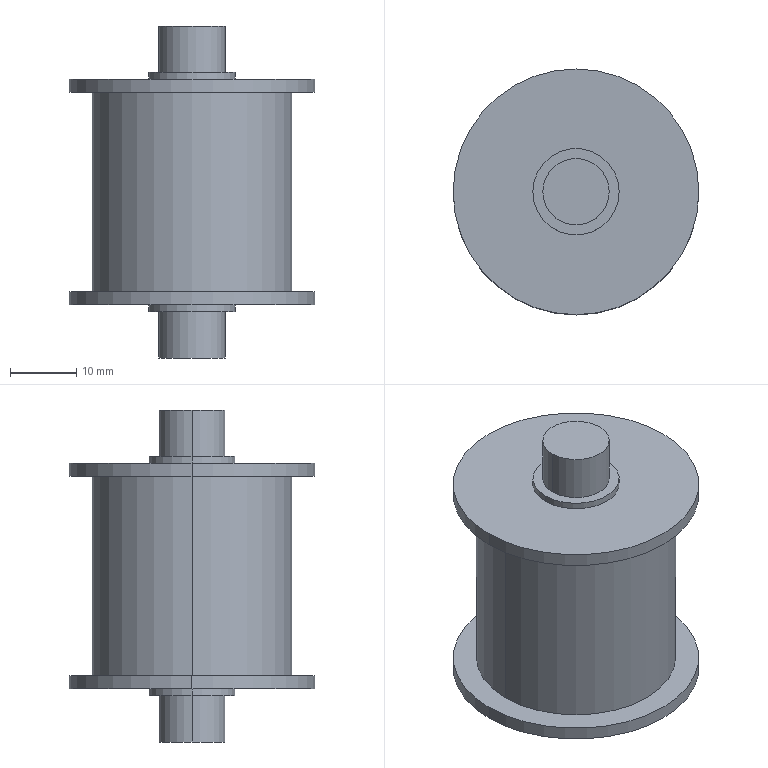Part | STEP file | (PA01.001.LX015) Idler A | 1 solid | 22 faces | box 37 x 37 x 50 mm | volume 26872 mm3 | cylinder 14 | plane 8 | commonest cylinder face diameters 10 x4 13 x4 37 x4 30 x2
STEP:
#1=CARTESIAN_POINT('',(0.,0.,0.));
#2=DIRECTION('',(0.,0.,1.));
#3=DIRECTION('',(1.,0.,0.));
#4=AXIS2_PLACEMENT_3D('',#1,#2,#3);
#5=CARTESIAN_POINT('',(5.,0.,25.));
#6=VERTEX_POINT('',#5);
#7=CARTESIAN_POINT('',(-5.,0.,25.));
#8=VERTEX_POINT('',#7);
#9=CARTESIAN_POINT('',(0.,0.,25.));
#10=DIRECTION('',(0.,0.,1.));
#11=DIRECTION('',(1.,0.,0.));
#12=AXIS2_PLACEMENT_3D('',#9,#10,#11);
#13=CIRCLE('',#12,5.);
#14=CARTESIAN_POINT('',(0.,0.,25.));
#15=DIRECTION('',(0.,0.,-1.));
#16=DIRECTION('',(-1.,0.,0.));
#17=AXIS2_PLACEMENT_3D('',#14,#15,#16);
#18=CYLINDRICAL_SURFACE('',#17,5.);
#19=CARTESIAN_POINT('',(3.142,0.));
#20=DIRECTION('',(-1.,0.));
#21=VECTOR('',#20,1.);
#22=LINE('',#19,#21);
#23=(GEOMETRIC_REPRESENTATION_CONTEXT(2)PARAMETRIC_REPRESENTATION_CONTEXT()REPRESENTATION_CONTEXT('',''));
#24=DEFINITIONAL_REPRESENTATION('',(#22),#23);
#25=PCURVE('',#18,#24);
#26=CARTESIAN_POINT('',(0.,0.,25.));
#27=DIRECTION('',(0.,0.,1.));
#28=DIRECTION('',(1.,0.,0.));
#29=AXIS2_PLACEMENT_3D('',#26,#27,#28);
#30=PLANE('',#29);
#31=CARTESIAN_POINT('',(0.,0.));
#32=DIRECTION('',(1.,0.));
#33=AXIS2_PLACEMENT_2D('',#31,#32);
#34=CIRCLE('',#33,5.);
#35=(GEOMETRIC_REPRESENTATION_CONTEXT(2)PARAMETRIC_REPRESENTATION_CONTEXT()REPRESENTATION_CONTEXT('',''));
#36=DEFINITIONAL_REPRESENTATION('',(#34),#35);
#37=PCURVE('',#30,#36);
#38=SURFACE_CURVE('',#13,(#25,#37),.PCURVE_S1.);
#39=EDGE_CURVE('',#6,#8,#38,.T.);
#40=ORIENTED_EDGE('',*,*,#39,.F.);
#41=CARTESIAN_POINT('',(5.,0.,18.));
#42=VERTEX_POINT('',#41);
#43=CARTESIAN_POINT('',(5.,0.,25.));
#44=DIRECTION('',(0.,0.,-1.));
#45=VECTOR('',#44,1.);
#46=LINE('',#43,#45);
#47=CARTESIAN_POINT('',(3.142,0.));
#48=DIRECTION('',(0.,1.));
#49=VECTOR('',#48,1.);
#50=LINE('',#47,#49);
#51=(GEOMETRIC_REPRESENTATION_CONTEXT(2)PARAMETRIC_REPRESENTATION_CONTEXT()REPRESENTATION_CONTEXT('',''));
#52=DEFINITIONAL_REPRESENTATION('',(#50),#51);
#53=PCURVE('',#18,#52);
#54=CARTESIAN_POINT('',(0.,0.,25.));
#55=DIRECTION('',(0.,0.,-1.));
#56=DIRECTION('',(-1.,0.,0.));
#57=AXIS2_PLACEMENT_3D('',#54,#55,#56);
#58=CYLINDRICAL_SURFACE('',#57,5.);
#59=CARTESIAN_POINT('',(3.142,0.));
#60=DIRECTION('',(0.,1.));
#61=VECTOR('',#60,1.);
#62=LINE('',#59,#61);
#63=(GEOMETRIC_REPRESENTATION_CONTEXT(2)PARAMETRIC_REPRESENTATION_CONTEXT()REPRESENTATION_CONTEXT('',''));
#64=DEFINITIONAL_REPRESENTATION('',(#62),#63);
#65=PCURVE('',#58,#64);
#66=SURFACE_CURVE('',#46,(#53,#65),.PCURVE_S1.);
#67=EDGE_CURVE('',#6,#42,#66,.T.);
#68=ORIENTED_EDGE('',*,*,#67,.T.);
#69=CARTESIAN_POINT('',(-5.,0.,18.));
#70=VERTEX_POINT('',#69);
#71=CARTESIAN_POINT('',(0.,0.,18.));
#72=DIRECTION('',(0.,0.,1.));
#73=DIRECTION('',(1.,0.,0.));
#74=AXIS2_PLACEMENT_3D('',#71,#72,#73);
#75=CIRCLE('',#74,5.);
#76=CARTESIAN_POINT('',(3.142,7.));
#77=DIRECTION('',(-1.,0.));
#78=VECTOR('',#77,1.);
#79=LINE('',#76,#78);
#80=(GEOMETRIC_REPRESENTATION_CONTEXT(2)PARAMETRIC_REPRESENTATION_CONTEXT()REPRESENTATION_CONTEXT('',''));
#81=DEFINITIONAL_REPRESENTATION('',(#79),#80);
#82=PCURVE('',#18,#81);
#83=CARTESIAN_POINT('',(0.,0.,18.));
#84=DIRECTION('',(0.,0.,1.));
#85=DIRECTION('',(1.,0.,0.));
#86=AXIS2_PLACEMENT_3D('',#83,#84,#85);
#87=PLANE('',#86);
#88=CARTESIAN_POINT('',(0.,0.));
#89=DIRECTION('',(1.,0.));
#90=AXIS2_PLACEMENT_2D('',#88,#89);
#91=CIRCLE('',#90,5.);
#92=(GEOMETRIC_REPRESENTATION_CONTEXT(2)PARAMETRIC_REPRESENTATION_CONTEXT()REPRESENTATION_CONTEXT('',''));
#93=DEFINITIONAL_REPRESENTATION('',(#91),#92);
#94=PCURVE('',#87,#93);
#95=SURFACE_CURVE('',#75,(#82,#94),.PCURVE_S1.);
#96=EDGE_CURVE('',#42,#70,#95,.T.);
#97=ORIENTED_EDGE('',*,*,#96,.T.);
#98=CARTESIAN_POINT('',(-5.,0.,25.));
#99=DIRECTION('',(0.,0.,-1.));
#100=VECTOR('',#99,1.);
#101=LINE('',#98,#100);
#102=CARTESIAN_POINT('',(0.,0.));
#103=DIRECTION('',(0.,1.));
#104=VECTOR('',#103,1.);
#105=LINE('',#102,#104);
#106=(GEOMETRIC_REPRESENTATION_CONTEXT(2)PARAMETRIC_REPRESENTATION_CONTEXT()REPRESENTATION_CONTEXT('',''));
#107=DEFINITIONAL_REPRESENTATION('',(#105),#106);
#108=PCURVE('',#18,#107);
#109=CARTESIAN_POINT('',(6.283,0.));
#110=DIRECTION('',(0.,1.));
#111=VECTOR('',#110,1.);
#112=LINE('',#109,#111);
#113=(GEOMETRIC_REPRESENTATION_CONTEXT(2)PARAMETRIC_REPRESENTATION_CONTEXT()REPRESENTATION_CONTEXT('',''));
#114=DEFINITIONAL_REPRESENTATION('',(#112),#113);
#115=PCURVE('',#58,#114);
#116=SURFACE_CURVE('',#101,(#108,#115),.PCURVE_S1.);
#117=EDGE_CURVE('',#8,#70,#116,.T.);
#118=ORIENTED_EDGE('',*,*,#117,.F.);
#119=EDGE_LOOP('',(#40,#68,#97,#118));
#120=FACE_BOUND('',#119,.T.);
#121=ADVANCED_FACE('',(#120),#18,.T.);
#122=CARTESIAN_POINT('',(6.5,0.,18.));
#123=VERTEX_POINT('',#122);
#124=CARTESIAN_POINT('',(-6.5,0.,18.));
#125=VERTEX_POINT('',#124);
#126=CARTESIAN_POINT('',(0.,0.,18.));
#127=DIRECTION('',(0.,0.,1.));
#128=DIRECTION('',(1.,0.,0.));
#129=AXIS2_PLACEMENT_3D('',#126,#127,#128);
#130=CIRCLE('',#129,6.5);
#131=CARTESIAN_POINT('',(0.,0.,18.));
#132=DIRECTION('',(0.,0.,-1.));
#133=DIRECTION('',(-1.,0.,0.));
#134=AXIS2_PLACEMENT_3D('',#131,#132,#133);
#135=CYLINDRICAL_SURFACE('',#134,6.5);
#136=CARTESIAN_POINT('',(3.142,0.));
#137=DIRECTION('',(-1.,0.));
#138=VECTOR('',#137,1.);
#139=LINE('',#136,#138);
#140=(GEOMETRIC_REPRESENTATION_CONTEXT(2)PARAMETRIC_REPRESENTATION_CONTEXT()REPRESENTATION_CONTEXT('',''));
#141=DEFINITIONAL_REPRESENTATION('',(#139),#140);
#142=PCURVE('',#135,#141);
#143=CARTESIAN_POINT('',(0.,0.));
#144=DIRECTION('',(1.,0.));
#145=AXIS2_PLACEMENT_2D('',#143,#144);
#146=CIRCLE('',#145,6.5);
#147=(GEOMETRIC_REPRESENTATION_CONTEXT(2)PARAMETRIC_REPRESENTATION_CONTEXT()REPRESENTATION_CONTEXT('',''));
#148=DEFINITIONAL_REPRESENTATION('',(#146),#147);
#149=PCURVE('',#87,#148);
#150=SURFACE_CURVE('',#130,(#142,#149),.PCURVE_S1.);
#151=EDGE_CURVE('',#123,#125,#150,.T.);
#152=ORIENTED_EDGE('',*,*,#151,.F.);
#153=CARTESIAN_POINT('',(6.5,0.,17.));
#154=VERTEX_POINT('',#153);
#155=CARTESIAN_POINT('',(6.5,0.,18.));
#156=DIRECTION('',(0.,0.,-1.));
#157=VECTOR('',#156,1.);
#158=LINE('',#155,#157);
#159=CARTESIAN_POINT('',(3.142,0.));
#160=DIRECTION('',(0.,1.));
#161=VECTOR('',#160,1.);
#162=LINE('',#159,#161);
#163=(GEOMETRIC_REPRESENTATION_CONTEXT(2)PARAMETRIC_REPRESENTATION_CONTEXT()REPRESENTATION_CONTEXT('',''));
#164=DEFINITIONAL_REPRESENTATION('',(#162),#163);
#165=PCURVE('',#135,#164);
#166=CARTESIAN_POINT('',(0.,0.,18.));
#167=DIRECTION('',(0.,0.,-1.));
#168=DIRECTION('',(-1.,0.,0.));
#169=AXIS2_PLACEMENT_3D('',#166,#167,#168);
#170=CYLINDRICAL_SURFACE('',#169,6.5);
#171=CARTESIAN_POINT('',(3.142,0.));
#172=DIRECTION('',(0.,1.));
#173=VECTOR('',#172,1.);
#174=LINE('',#171,#173);
#175=(GEOMETRIC_REPRESENTATION_CONTEXT(2)PARAMETRIC_REPRESENTATION_CONTEXT()REPRESENTATION_CONTEXT('',''));
#176=DEFINITIONAL_REPRESENTATION('',(#174),#175);
#177=PCURVE('',#170,#176);
#178=SURFACE_CURVE('',#158,(#165,#177),.PCURVE_S1.);
#179=EDGE_CURVE('',#123,#154,#178,.T.);
#180=ORIENTED_EDGE('',*,*,#179,.T.);
#181=CARTESIAN_POINT('',(-6.5,0.,17.));
#182=VERTEX_POINT('',#181);
#183=CARTESIAN_POINT('',(0.,0.,17.));
#184=DIRECTION('',(0.,0.,1.));
#185=DIRECTION('',(1.,0.,0.));
#186=AXIS2_PLACEMENT_3D('',#183,#184,#185);
#187=CIRCLE('',#186,6.5);
#188=CARTESIAN_POINT('',(3.142,1.));
#189=DIRECTION('',(-1.,0.));
#190=VECTOR('',#189,1.);
#191=LINE('',#188,#190);
#192=(GEOMETRIC_REPRESENTATION_CONTEXT(2)PARAMETRIC_REPRESENTATION_CONTEXT()REPRESENTATION_CONTEXT('',''));
#193=DEFINITIONAL_REPRESENTATION('',(#191),#192);
#194=PCURVE('',#135,#193);
#195=CARTESIAN_POINT('',(0.,0.,17.));
#196=DIRECTION('',(0.,0.,1.));
#197=DIRECTION('',(1.,0.,0.));
#198=AXIS2_PLACEMENT_3D('',#195,#196,#197);
#199=PLANE('',#198);
#200=CARTESIAN_POINT('',(0.,0.));
#201=DIRECTION('',(1.,0.));
#202=AXIS2_PLACEMENT_2D('',#200,#201);
#203=CIRCLE('',#202,6.5);
#204=(GEOMETRIC_REPRESENTATION_CONTEXT(2)PARAMETRIC_REPRESENTATION_CONTEXT()REPRESENTATION_CONTEXT('',''));
#205=DEFINITIONAL_REPRESENTATION('',(#203),#204);
#206=PCURVE('',#199,#205);
#207=SURFACE_CURVE('',#187,(#194,#206),.PCURVE_S1.);
#208=EDGE_CURVE('',#154,#182,#207,.T.);
#209=ORIENTED_EDGE('',*,*,#208,.T.);
#210=CARTESIAN_POINT('',(-6.5,0.,18.));
#211=DIRECTION('',(0.,0.,-1.));
#212=VECTOR('',#211,1.);
#213=LINE('',#210,#212);
#214=CARTESIAN_POINT('',(0.,0.));
#215=DIRECTION('',(0.,1.));
#216=VECTOR('',#215,1.);
#217=LINE('',#214,#216);
#218=(GEOMETRIC_REPRESENTATION_CONTEXT(2)PARAMETRIC_REPRESENTATION_CONTEXT()REPRESENTATION_CONTEXT('',''));
#219=DEFINITIONAL_REPRESENTATION('',(#217),#218);
#220=PCURVE('',#135,#219);
#221=CARTESIAN_POINT('',(6.283,0.));
#222=DIRECTION('',(0.,1.));
#223=VECTOR('',#222,1.);
#224=LINE('',#221,#223);
#225=(GEOMETRIC_REPRESENTATION_CONTEXT(2)PARAMETRIC_REPRESENTATION_CONTEXT()REPRESENTATION_CONTEXT('',''));
#226=DEFINITIONAL_REPRESENTATION('',(#224),#225);
#227=PCURVE('',#170,#226);
#228=SURFACE_CURVE('',#213,(#220,#227),.PCURVE_S1.);
#229=EDGE_CURVE('',#125,#182,#228,.T.);
#230=ORIENTED_EDGE('',*,*,#229,.F.);
#231=EDGE_LOOP('',(#152,#180,#209,#230));
#232=FACE_BOUND('',#231,.T.);
#233=ADVANCED_FACE('',(#232),#135,.T.);
#234=CARTESIAN_POINT('',(-5.,0.,-25.));
#235=VERTEX_POINT('',#234);
#236=CARTESIAN_POINT('',(5.,0.,-25.));
#237=VERTEX_POINT('',#236);
#238=CARTESIAN_POINT('',(0.,0.,-25.));
#239=DIRECTION('',(0.,0.,-1.));
#240=DIRECTION('',(-1.,0.,0.));
#241=AXIS2_PLACEMENT_3D('',#238,#239,#240);
#242=CIRCLE('',#241,5.);
#243=CARTESIAN_POINT('',(0.,0.,-25.));
#244=DIRECTION('',(0.,0.,1.));
#245=DIRECTION('',(1.,0.,0.));
#246=AXIS2_PLACEMENT_3D('',#243,#244,#245);
#247=CYLINDRICAL_SURFACE('',#246,5.);
#248=CARTESIAN_POINT('',(3.142,0.));
#249=DIRECTION('',(-1.,0.));
#250=VECTOR('',#249,1.);
#251=LINE('',#248,#250);
#252=(GEOMETRIC_REPRESENTATION_CONTEXT(2)PARAMETRIC_REPRESENTATION_CONTEXT()REPRESENTATION_CONTEXT('',''));
#253=DEFINITIONAL_REPRESENTATION('',(#251),#252);
#254=PCURVE('',#247,#253);
#255=CARTESIAN_POINT('',(0.,0.,-25.));
#256=DIRECTION('',(0.,0.,-1.));
#257=DIRECTION('',(-1.,0.,0.));
#258=AXIS2_PLACEMENT_3D('',#255,#256,#257);
#259=PLANE('',#258);
#260=CARTESIAN_POINT('',(0.,0.));
#261=DIRECTION('',(1.,0.));
#262=AXIS2_PLACEMENT_2D('',#260,#261);
#263=CIRCLE('',#262,5.);
#264=(GEOMETRIC_REPRESENTATION_CONTEXT(2)PARAMETRIC_REPRESENTATION_CONTEXT()REPRESENTATION_CONTEXT('',''));
#265=DEFINITIONAL_REPRESENTATION('',(#263),#264);
#266=PCURVE('',#259,#265);
#267=SURFACE_CURVE('',#242,(#254,#266),.PCURVE_S1.);
#268=EDGE_CURVE('',#235,#237,#267,.T.);
#269=ORIENTED_EDGE('',*,*,#268,.F.);
#270=CARTESIAN_POINT('',(-5.,0.,-18.));
#271=VERTEX_POINT('',#270);
#272=CARTESIAN_POINT('',(-5.,0.,-25.));
#273=DIRECTION('',(0.,0.,1.));
#274=VECTOR('',#273,1.);
#275=LINE('',#272,#274);
#276=CARTESIAN_POINT('',(3.142,0.));
#277=DIRECTION('',(0.,1.));
#278=VECTOR('',#277,1.);
#279=LINE('',#276,#278);
#280=(GEOMETRIC_REPRESENTATION_CONTEXT(2)PARAMETRIC_REPRESENTATION_CONTEXT()REPRESENTATION_CONTEXT('',''));
#281=DEFINITIONAL_REPRESENTATION('',(#279),#280);
#282=PCURVE('',#247,#281);
#283=CARTESIAN_POINT('',(0.,0.,-25.));
#284=DIRECTION('',(0.,0.,1.));
#285=DIRECTION('',(1.,0.,0.));
#286=AXIS2_PLACEMENT_3D('',#283,#284,#285);
#287=CYLINDRICAL_SURFACE('',#286,5.);
#288=CARTESIAN_POINT('',(3.142,0.));
#289=DIRECTION('',(0.,1.));
#290=VECTOR('',#289,1.);
#291=LINE('',#288,#290);
#292=(GEOMETRIC_REPRESENTATION_CONTEXT(2)PARAMETRIC_REPRESENTATION_CONTEXT()REPRESENTATION_CONTEXT('',''));
#293=DEFINITIONAL_REPRESENTATION('',(#291),#292);
#294=PCURVE('',#287,#293);
#295=SURFACE_CURVE('',#275,(#282,#294),.PCURVE_S1.);
#296=EDGE_CURVE('',#235,#271,#295,.T.);
#297=ORIENTED_EDGE('',*,*,#296,.T.);
#298=CARTESIAN_POINT('',(5.,0.,-18.));
#299=VERTEX_POINT('',#298);
#300=CARTESIAN_POINT('',(0.,0.,-18.));
#301=DIRECTION('',(0.,0.,-1.));
#302=DIRECTION('',(-1.,0.,0.));
#303=AXIS2_PLACEMENT_3D('',#300,#301,#302);
#304=CIRCLE('',#303,5.);
#305=CARTESIAN_POINT('',(3.142,7.));
#306=DIRECTION('',(-1.,0.));
#307=VECTOR('',#306,1.);
#308=LINE('',#305,#307);
#309=(GEOMETRIC_REPRESENTATION_CONTEXT(2)PARAMETRIC_REPRESENTATION_CONTEXT()REPRESENTATION_CONTEXT('',''));
#310=DEFINITIONAL_REPRESENTATION('',(#308),#309);
#311=PCURVE('',#247,#310);
#312=CARTESIAN_POINT('',(0.,0.,-18.));
#313=DIRECTION('',(0.,0.,-1.));
#314=DIRECTION('',(-1.,0.,0.));
#315=AXIS2_PLACEMENT_3D('',#312,#313,#314);
#316=PLANE('',#315);
#317=CARTESIAN_POINT('',(0.,0.));
#318=DIRECTION('',(1.,0.));
#319=AXIS2_PLACEMENT_2D('',#317,#318);
#320=CIRCLE('',#319,5.);
#321=(GEOMETRIC_REPRESENTATION_CONTEXT(2)PARAMETRIC_REPRESENTATION_CONTEXT()REPRESENTATION_CONTEXT('',''));
#322=DEFINITIONAL_REPRESENTATION('',(#320),#321);
#323=PCURVE('',#316,#322);
#324=SURFACE_CURVE('',#304,(#311,#323),.PCURVE_S1.);
#325=EDGE_CURVE('',#271,#299,#324,.T.);
#326=ORIENTED_EDGE('',*,*,#325,.T.);
#327=CARTESIAN_POINT('',(5.,0.,-25.));
#328=DIRECTION('',(0.,0.,1.));
#329=VECTOR('',#328,1.);
#330=LINE('',#327,#329);
#331=CARTESIAN_POINT('',(0.,0.));
#332=DIRECTION('',(0.,1.));
#333=VECTOR('',#332,1.);
#334=LINE('',#331,#333);
#335=(GEOMETRIC_REPRESENTATION_CONTEXT(2)PARAMETRIC_REPRESENTATION_CONTEXT()REPRESENTATION_CONTEXT('',''));
#336=DEFINITIONAL_REPRESENTATION('',(#334),#335);
#337=PCURVE('',#247,#336);
#338=CARTESIAN_POINT('',(6.283,0.));
#339=DIRECTION('',(0.,1.));
#340=VECTOR('',#339,1.);
#341=LINE('',#338,#340);
#342=(GEOMETRIC_REPRESENTATION_CONTEXT(2)PARAMETRIC_REPRESENTATION_CONTEXT()REPRESENTATION_CONTEXT('',''));
#343=DEFINITIONAL_REPRESENTATION('',(#341),#342);
#344=PCURVE('',#287,#343);
#345=SURFACE_CURVE('',#330,(#337,#344),.PCURVE_S1.);
#346=EDGE_CURVE('',#237,#299,#345,.T.);
#347=ORIENTED_EDGE('',*,*,#346,.F.);
#348=EDGE_LOOP('',(#269,#297,#326,#347));
#349=FACE_BOUND('',#348,.T.);
#350=ADVANCED_FACE('',(#349),#247,.T.);
#351=CARTESIAN_POINT('',(-6.5,0.,-18.));
#352=VERTEX_POINT('',#351);
#353=CARTESIAN_POINT('',(6.5,0.,-18.));
#354=VERTEX_POINT('',#353);
#355=CARTESIAN_POINT('',(0.,0.,-18.));
#356=DIRECTION('',(0.,0.,-1.));
#357=DIRECTION('',(-1.,0.,0.));
#358=AXIS2_PLACEMENT_3D('',#355,#356,#357);
#359=CIRCLE('',#358,6.5);
#360=CARTESIAN_POINT('',(0.,0.,-18.));
#361=DIRECTION('',(0.,0.,1.));
#362=DIRECTION('',(1.,0.,0.));
#363=AXIS2_PLACEMENT_3D('',#360,#361,#362);
#364=CYLINDRICAL_SURFACE('',#363,6.5);
#365=CARTESIAN_POINT('',(3.142,0.));
#366=DIRECTION('',(-1.,0.));
#367=VECTOR('',#366,1.);
#368=LINE('',#365,#367);
#369=(GEOMETRIC_REPRESENTATION_CONTEXT(2)PARAMETRIC_REPRESENTATION_CONTEXT()REPRESENTATION_CONTEXT('',''));
#370=DEFINITIONAL_REPRESENTATION('',(#368),#369);
#371=PCURVE('',#364,#370);
#372=CARTESIAN_POINT('',(0.,0.));
#373=DIRECTION('',(1.,0.));
#374=AXIS2_PLACEMENT_2D('',#372,#373);
#375=CIRCLE('',#374,6.5);
#376=(GEOMETRIC_REPRESENTATION_CONTEXT(2)PARAMETRIC_REPRESENTATION_CONTEXT()REPRESENTATION_CONTEXT('',''));
#377=DEFINITIONAL_REPRESENTATION('',(#375),#376);
#378=PCURVE('',#316,#377);
#379=SURFACE_CURVE('',#359,(#371,#378),.PCURVE_S1.);
#380=EDGE_CURVE('',#352,#354,#379,.T.);
#381=ORIENTED_EDGE('',*,*,#380,.F.);
#382=CARTESIAN_POINT('',(-6.5,0.,-17.));
#383=VERTEX_POINT('',#382);
#384=CARTESIAN_POINT('',(-6.5,0.,-18.));
#385=DIRECTION('',(0.,0.,1.));
#386=VECTOR('',#385,1.);
#387=LINE('',#384,#386);
#388=CARTESIAN_POINT('',(3.142,0.));
#389=DIRECTION('',(0.,1.));
#390=VECTOR('',#389,1.);
#391=LINE('',#388,#390);
#392=(GEOMETRIC_REPRESENTATION_CONTEXT(2)PARAMETRIC_REPRESENTATION_CONTEXT()REPRESENTATION_CONTEXT('',''));
#393=DEFINITIONAL_REPRESENTATION('',(#391),#392);
#394=PCURVE('',#364,#393);
#395=CARTESIAN_POINT('',(0.,0.,-18.));
#396=DIRECTION('',(0.,0.,1.));
#397=DIRECTION('',(1.,0.,0.));
#398=AXIS2_PLACEMENT_3D('',#395,#396,#397);
#399=CYLINDRICAL_SURFACE('',#398,6.5);
#400=CARTESIAN_POINT('',(3.142,0.));
#401=DIRECTION('',(0.,1.));
#402=VECTOR('',#401,1.);
#403=LINE('',#400,#402);
#404=(GEOMETRIC_REPRESENTATION_CONTEXT(2)PARAMETRIC_REPRESENTATION_CONTEXT()REPRESENTATION_CONTEXT('',''));
#405=DEFINITIONAL_REPRESENTATION('',(#403),#404);
#406=PCURVE('',#399,#405);
#407=SURFACE_CURVE('',#387,(#394,#406),.PCURVE_S1.);
#408=EDGE_CURVE('',#352,#383,#407,.T.);
#409=ORIENTED_EDGE('',*,*,#408,.T.);
#410=CARTESIAN_POINT('',(6.5,0.,-17.));
#411=VERTEX_POINT('',#410);
#412=CARTESIAN_POINT('',(0.,0.,-17.));
#413=DIRECTION('',(0.,0.,-1.));
#414=DIRECTION('',(-1.,0.,0.));
#415=AXIS2_PLACEMENT_3D('',#412,#413,#414);
#416=CIRCLE('',#415,6.5);
#417=CARTESIAN_POINT('',(3.142,1.));
#418=DIRECTION('',(-1.,0.));
#419=VECTOR('',#418,1.);
#420=LINE('',#417,#419);
#421=(GEOMETRIC_REPRESENTATION_CONTEXT(2)PARAMETRIC_REPRESENTATION_CONTEXT()REPRESENTATION_CONTEXT('',''));
#422=DEFINITIONAL_REPRESENTATION('',(#420),#421);
#423=PCURVE('',#364,#422);
#424=CARTESIAN_POINT('',(0.,0.,-17.));
#425=DIRECTION('',(0.,0.,-1.));
#426=DIRECTION('',(-1.,0.,0.));
#427=AXIS2_PLACEMENT_3D('',#424,#425,#426);
#428=PLANE('',#427);
#429=CARTESIAN_POINT('',(0.,0.));
#430=DIRECTION('',(1.,0.));
#431=AXIS2_PLACEMENT_2D('',#429,#430);
#432=CIRCLE('',#431,6.5);
#433=(GEOMETRIC_REPRESENTATION_CONTEXT(2)PARAMETRIC_REPRESENTATION_CONTEXT()REPRESENTATION_CONTEXT('',''));
#434=DEFINITIONAL_REPRESENTATION('',(#432),#433);
#435=PCURVE('',#428,#434);
#436=SURFACE_CURVE('',#416,(#423,#435),.PCURVE_S1.);
#437=EDGE_CURVE('',#383,#411,#436,.T.);
#438=ORIENTED_EDGE('',*,*,#437,.T.);
#439=CARTESIAN_POINT('',(6.5,0.,-18.));
#440=DIRECTION('',(0.,0.,1.));
#441=VECTOR('',#440,1.);
#442=LINE('',#439,#441);
#443=CARTESIAN_POINT('',(0.,0.));
#444=DIRECTION('',(0.,1.));
#445=VECTOR('',#444,1.);
#446=LINE('',#443,#445);
#447=(GEOMETRIC_REPRESENTATION_CONTEXT(2)PARAMETRIC_REPRESENTATION_CONTEXT()REPRESENTATION_CONTEXT('',''));
#448=DEFINITIONAL_REPRESENTATION('',(#446),#447);
#449=PCURVE('',#364,#448);
#450=CARTESIAN_POINT('',(6.283,0.));
#451=DIRECTION('',(0.,1.));
#452=VECTOR('',#451,1.);
#453=LINE('',#450,#452);
#454=(GEOMETRIC_REPRESENTATION_CONTEXT(2)PARAMETRIC_REPRESENTATION_CONTEXT()REPRESENTATION_CONTEXT('',''));
#455=DEFINITIONAL_REPRESENTATION('',(#453),#454);
#456=PCURVE('',#399,#455);
#457=SURFACE_CURVE('',#442,(#449,#456),.PCURVE_S1.);
#458=EDGE_CURVE('',#354,#411,#457,.T.);
#459=ORIENTED_EDGE('',*,*,#458,.F.);
#460=EDGE_LOOP('',(#381,#409,#438,#459));
#461=FACE_BOUND('',#460,.T.);
#462=ADVANCED_FACE('',(#461),#364,.T.);
#463=CARTESIAN_POINT('',(-18.5,0.,-17.));
#464=VERTEX_POINT('',#463);
#465=CARTESIAN_POINT('',(18.5,0.,-17.));
#466=VERTEX_POINT('',#465);
#467=CARTESIAN_POINT('',(0.,0.,-17.));
#468=DIRECTION('',(0.,0.,-1.));
#469=DIRECTION('',(-1.,0.,0.));
#470=AXIS2_PLACEMENT_3D('',#467,#468,#469);
#471=CIRCLE('',#470,18.5);
#472=CARTESIAN_POINT('',(0.,0.,-17.));
#473=DIRECTION('',(0.,0.,1.));
#474=DIRECTION('',(1.,0.,0.));
#475=AXIS2_PLACEMENT_3D('',#472,#473,#474);
#476=CYLINDRICAL_SURFACE('',#475,18.5);
#477=CARTESIAN_POINT('',(3.142,0.));
#478=DIRECTION('',(-1.,0.));
#479=VECTOR('',#478,1.);
#480=LINE('',#477,#479);
#481=(GEOMETRIC_REPRESENTATION_CONTEXT(2)PARAMETRIC_REPRESENTATION_CONTEXT()REPRESENTATION_CONTEXT('',''));
#482=DEFINITIONAL_REPRESENTATION('',(#480),#481);
#483=PCURVE('',#476,#482);
#484=CARTESIAN_POINT('',(0.,0.));
#485=DIRECTION('',(1.,0.));
#486=AXIS2_PLACEMENT_2D('',#484,#485);
#487=CIRCLE('',#486,18.5);
#488=(GEOMETRIC_REPRESENTATION_CONTEXT(2)PARAMETRIC_REPRESENTATION_CONTEXT()REPRESENTATION_CONTEXT('',''));
#489=DEFINITIONAL_REPRESENTATION('',(#487),#488);
#490=PCURVE('',#428,#489);
#491=SURFACE_CURVE('',#471,(#483,#490),.PCURVE_S1.);
#492=EDGE_CURVE('',#464,#466,#491,.T.);
#493=ORIENTED_EDGE('',*,*,#492,.F.);
#494=CARTESIAN_POINT('',(-18.5,0.,-15.));
#495=VERTEX_POINT('',#494);
#496=CARTESIAN_POINT('',(-18.5,0.,-17.));
#497=DIRECTION('',(0.,0.,1.));
#498=VECTOR('',#497,1.);
#499=LINE('',#496,#498);
#500=CARTESIAN_POINT('',(3.142,0.));
#501=DIRECTION('',(0.,1.));
#502=VECTOR('',#501,1.);
#503=LINE('',#500,#502);
#504=(GEOMETRIC_REPRESENTATION_CONTEXT(2)PARAMETRIC_REPRESENTATION_CONTEXT()REPRESENTATION_CONTEXT('',''));
#505=DEFINITIONAL_REPRESENTATION('',(#503),#504);
#506=PCURVE('',#476,#505);
#507=CARTESIAN_POINT('',(0.,0.,-17.));
#508=DIRECTION('',(0.,0.,1.));
#509=DIRECTION('',(1.,0.,0.));
#510=AXIS2_PLACEMENT_3D('',#507,#508,#509);
#511=CYLINDRICAL_SURFACE('',#510,18.5);
#512=CARTESIAN_POINT('',(3.142,0.));
#513=DIRECTION('',(0.,1.));
#514=VECTOR('',#513,1.);
#515=LINE('',#512,#514);
#516=(GEOMETRIC_REPRESENTATION_CONTEXT(2)PARAMETRIC_REPRESENTATION_CONTEXT()REPRESENTATION_CONTEXT('',''));
#517=DEFINITIONAL_REPRESENTATION('',(#515),#516);
#518=PCURVE('',#511,#517);
#519=SURFACE_CURVE('',#499,(#506,#518),.PCURVE_S1.);
#520=EDGE_CURVE('',#464,#495,#519,.T.);
#521=ORIENTED_EDGE('',*,*,#520,.T.);
#522=CARTESIAN_POINT('',(18.5,0.,-15.));
#523=VERTEX_POINT('',#522);
#524=CARTESIAN_POINT('',(0.,0.,-15.));
#525=DIRECTION('',(0.,0.,-1.));
#526=DIRECTION('',(-1.,0.,0.));
#527=AXIS2_PLACEMENT_3D('',#524,#525,#526);
#528=CIRCLE('',#527,18.5);
#529=CARTESIAN_POINT('',(3.142,2.));
#530=DIRECTION('',(-1.,0.));
#531=VECTOR('',#530,1.);
#532=LINE('',#529,#531);
#533=(GEOMETRIC_REPRESENTATION_CONTEXT(2)PARAMETRIC_REPRESENTATION_CONTEXT()REPRESENTATION_CONTEXT('',''));
#534=DEFINITIONAL_REPRESENTATION('',(#532),#533);
#535=PCURVE('',#476,#534);
#536=CARTESIAN_POINT('',(0.,0.,-15.));
#537=DIRECTION('',(0.,0.,-1.));
#538=DIRECTION('',(-1.,0.,0.));
#539=AXIS2_PLACEMENT_3D('',#536,#537,#538);
#540=PLANE('',#539);
#541=CARTESIAN_POINT('',(0.,0.));
#542=DIRECTION('',(1.,0.));
#543=AXIS2_PLACEMENT_2D('',#541,#542);
#544=CIRCLE('',#543,18.5);
#545=(GEOMETRIC_REPRESENTATION_CONTEXT(2)PARAMETRIC_REPRESENTATION_CONTEXT()REPRESENTATION_CONTEXT('',''));
#546=DEFINITIONAL_REPRESENTATION('',(#544),#545);
#547=PCURVE('',#540,#546);
#548=SURFACE_CURVE('',#528,(#535,#547),.PCURVE_S1.);
#549=EDGE_CURVE('',#495,#523,#548,.T.);
#550=ORIENTED_EDGE('',*,*,#549,.T.);
#551=CARTESIAN_POINT('',(18.5,0.,-17.));
#552=DIRECTION('',(0.,0.,1.));
#553=VECTOR('',#552,1.);
#554=LINE('',#551,#553);
#555=CARTESIAN_POINT('',(0.,0.));
#556=DIRECTION('',(0.,1.));
#557=VECTOR('',#556,1.);
#558=LINE('',#555,#557);
#559=(GEOMETRIC_REPRESENTATION_CONTEXT(2)PARAMETRIC_REPRESENTATION_CONTEXT()REPRESENTATION_CONTEXT('',''));
#560=DEFINITIONAL_REPRESENTATION('',(#558),#559);
#561=PCURVE('',#476,#560);
#562=CARTESIAN_POINT('',(6.283,0.));
#563=DIRECTION('',(0.,1.));
#564=VECTOR('',#563,1.);
#565=LINE('',#562,#564);
#566=(GEOMETRIC_REPRESENTATION_CONTEXT(2)PARAMETRIC_REPRESENTATION_CONTEXT()REPRESENTATION_CONTEXT('',''));
#567=DEFINITIONAL_REPRESENTATION('',(#565),#566);
#568=PCURVE('',#511,#567);
#569=SURFACE_CURVE('',#554,(#561,#568),.PCURVE_S1.);
#570=EDGE_CURVE('',#466,#523,#569,.T.);
#571=ORIENTED_EDGE('',*,*,#570,.F.);
#572=EDGE_LOOP('',(#493,#521,#550,#571));
#573=FACE_BOUND('',#572,.T.);
#574=ADVANCED_FACE('',(#573),#476,.T.);
#575=CARTESIAN_POINT('',(18.5,0.,17.));
#576=VERTEX_POINT('',#575);
#577=CARTESIAN_POINT('',(-18.5,0.,17.));
#578=VERTEX_POINT('',#577);
#579=CARTESIAN_POINT('',(0.,0.,17.));
#580=DIRECTION('',(0.,0.,1.));
#581=DIRECTION('',(1.,0.,0.));
#582=AXIS2_PLACEMENT_3D('',#579,#580,#581);
#583=CIRCLE('',#582,18.5);
#584=CARTESIAN_POINT('',(0.,0.,17.));
#585=DIRECTION('',(0.,0.,-1.));
#586=DIRECTION('',(-1.,0.,0.));
#587=AXIS2_PLACEMENT_3D('',#584,#585,#586);
#588=CYLINDRICAL_SURFACE('',#587,18.5);
#589=CARTESIAN_POINT('',(3.142,0.));
#590=DIRECTION('',(-1.,0.));
#591=VECTOR('',#590,1.);
#592=LINE('',#589,#591);
#593=(GEOMETRIC_REPRESENTATION_CONTEXT(2)PARAMETRIC_REPRESENTATION_CONTEXT()REPRESENTATION_CONTEXT('',''));
#594=DEFINITIONAL_REPRESENTATION('',(#592),#593);
#595=PCURVE('',#588,#594);
#596=CARTESIAN_POINT('',(0.,0.));
#597=DIRECTION('',(1.,0.));
#598=AXIS2_PLACEMENT_2D('',#596,#597);
#599=CIRCLE('',#598,18.5);
#600=(GEOMETRIC_REPRESENTATION_CONTEXT(2)PARAMETRIC_REPRESENTATION_CONTEXT()REPRESENTATION_CONTEXT('',''));
#601=DEFINITIONAL_REPRESENTATION('',(#599),#600);
#602=PCURVE('',#199,#601);
#603=SURFACE_CURVE('',#583,(#595,#602),.PCURVE_S1.);
#604=EDGE_CURVE('',#576,#578,#603,.T.);
#605=ORIENTED_EDGE('',*,*,#604,.F.);
#606=CARTESIAN_POINT('',(18.5,0.,15.));
#607=VERTEX_POINT('',#606);
#608=CARTESIAN_POINT('',(18.5,0.,17.));
#609=DIRECTION('',(0.,0.,-1.));
#610=VECTOR('',#609,1.);
#611=LINE('',#608,#610);
#612=CARTESIAN_POINT('',(3.142,0.));
#613=DIRECTION('',(0.,1.));
#614=VECTOR('',#613,1.);
#615=LINE('',#612,#614);
#616=(GEOMETRIC_REPRESENTATION_CONTEXT(2)PARAMETRIC_REPRESENTATION_CONTEXT()REPRESENTATION_CONTEXT('',''));
#617=DEFINITIONAL_REPRESENTATION('',(#615),#616);
#618=PCURVE('',#588,#617);
#619=CARTESIAN_POINT('',(0.,0.,17.));
#620=DIRECTION('',(0.,0.,-1.));
#621=DIRECTION('',(-1.,0.,0.));
#622=AXIS2_PLACEMENT_3D('',#619,#620,#621);
#623=CYLINDRICAL_SURFACE('',#622,18.5);
#624=CARTESIAN_POINT('',(3.142,0.));
#625=DIRECTION('',(0.,1.));
#626=VECTOR('',#625,1.);
#627=LINE('',#624,#626);
#628=(GEOMETRIC_REPRESENTATION_CONTEXT(2)PARAMETRIC_REPRESENTATION_CONTEXT()REPRESENTATION_CONTEXT('',''));
#629=DEFINITIONAL_REPRESENTATION('',(#627),#628);
#630=PCURVE('',#623,#629);
#631=SURFACE_CURVE('',#611,(#618,#630),.PCURVE_S1.);
#632=EDGE_CURVE('',#576,#607,#631,.T.);
#633=ORIENTED_EDGE('',*,*,#632,.T.);
#634=CARTESIAN_POINT('',(-18.5,0.,15.));
#635=VERTEX_POINT('',#634);
#636=CARTESIAN_POINT('',(0.,0.,15.));
#637=DIRECTION('',(0.,0.,1.));
#638=DIRECTION('',(1.,0.,0.));
#639=AXIS2_PLACEMENT_3D('',#636,#637,#638);
#640=CIRCLE('',#639,18.5);
#641=CARTESIAN_POINT('',(3.142,2.));
#642=DIRECTION('',(-1.,0.));
#643=VECTOR('',#642,1.);
#644=LINE('',#641,#643);
#645=(GEOMETRIC_REPRESENTATION_CONTEXT(2)PARAMETRIC_REPRESENTATION_CONTEXT()REPRESENTATION_CONTEXT('',''));
#646=DEFINITIONAL_REPRESENTATION('',(#644),#645);
#647=PCURVE('',#588,#646);
#648=CARTESIAN_POINT('',(0.,0.,15.));
#649=DIRECTION('',(0.,0.,1.));
#650=DIRECTION('',(1.,0.,0.));
#651=AXIS2_PLACEMENT_3D('',#648,#649,#650);
#652=PLANE('',#651);
#653=CARTESIAN_POINT('',(0.,0.));
#654=DIRECTION('',(1.,0.));
#655=AXIS2_PLACEMENT_2D('',#653,#654);
#656=CIRCLE('',#655,18.5);
#657=(GEOMETRIC_REPRESENTATION_CONTEXT(2)PARAMETRIC_REPRESENTATION_CONTEXT()REPRESENTATION_CONTEXT('',''));
#658=DEFINITIONAL_REPRESENTATION('',(#656),#657);
#659=PCURVE('',#652,#658);
#660=SURFACE_CURVE('',#640,(#647,#659),.PCURVE_S1.);
#661=EDGE_CURVE('',#607,#635,#660,.T.);
#662=ORIENTED_EDGE('',*,*,#661,.T.);
#663=CARTESIAN_POINT('',(-18.5,0.,17.));
#664=DIRECTION('',(0.,0.,-1.));
#665=VECTOR('',#664,1.);
#666=LINE('',#663,#665);
#667=CARTESIAN_POINT('',(0.,0.));
#668=DIRECTION('',(0.,1.));
#669=VECTOR('',#668,1.);
#670=LINE('',#667,#669);
#671=(GEOMETRIC_REPRESENTATION_CONTEXT(2)PARAMETRIC_REPRESENTATION_CONTEXT()REPRESENTATION_CONTEXT('',''));
#672=DEFINITIONAL_REPRESENTATION('',(#670),#671);
#673=PCURVE('',#588,#672);
#674=CARTESIAN_POINT('',(6.283,0.));
#675=DIRECTION('',(0.,1.));
#676=VECTOR('',#675,1.);
#677=LINE('',#674,#676);
#678=(GEOMETRIC_REPRESENTATION_CONTEXT(2)PARAMETRIC_REPRESENTATION_CONTEXT()REPRESENTATION_CONTEXT('',''));
#679=DEFINITIONAL_REPRESENTATION('',(#677),#678);
#680=PCURVE('',#623,#679);
#681=SURFACE_CURVE('',#666,(#673,#680),.PCURVE_S1.);
#682=EDGE_CURVE('',#578,#635,#681,.T.);
#683=ORIENTED_EDGE('',*,*,#682,.F.);
#684=EDGE_LOOP('',(#605,#633,#662,#683));
#685=FACE_BOUND('',#684,.T.);
#686=ADVANCED_FACE('',(#685),#588,.T.);
#687=CARTESIAN_POINT('',(15.,0.,15.));
#688=VERTEX_POINT('',#687);
#689=CARTESIAN_POINT('',(-15.,0.,15.));
#690=VERTEX_POINT('',#689);
#691=CARTESIAN_POINT('',(0.,0.,15.));
#692=DIRECTION('',(0.,0.,1.));
#693=DIRECTION('',(1.,0.,0.));
#694=AXIS2_PLACEMENT_3D('',#691,#692,#693);
#695=CIRCLE('',#694,15.);
#696=CARTESIAN_POINT('',(0.,0.,15.));
#697=DIRECTION('',(0.,0.,-1.));
#698=DIRECTION('',(-1.,0.,0.));
#699=AXIS2_PLACEMENT_3D('',#696,#697,#698);
#700=CYLINDRICAL_SURFACE('',#699,15.);
#701=CARTESIAN_POINT('',(3.142,0.));
#702=DIRECTION('',(-1.,0.));
#703=VECTOR('',#702,1.);
#704=LINE('',#701,#703);
#705=(GEOMETRIC_REPRESENTATION_CONTEXT(2)PARAMETRIC_REPRESENTATION_CONTEXT()REPRESENTATION_CONTEXT('',''));
#706=DEFINITIONAL_REPRESENTATION('',(#704),#705);
#707=PCURVE('',#700,#706);
#708=CARTESIAN_POINT('',(0.,0.));
#709=DIRECTION('',(1.,0.));
#710=AXIS2_PLACEMENT_2D('',#708,#709);
#711=CIRCLE('',#710,15.);
#712=(GEOMETRIC_REPRESENTATION_CONTEXT(2)PARAMETRIC_REPRESENTATION_CONTEXT()REPRESENTATION_CONTEXT('',''));
#713=DEFINITIONAL_REPRESENTATION('',(#711),#712);
#714=PCURVE('',#652,#713);
#715=SURFACE_CURVE('',#695,(#707,#714),.PCURVE_S1.);
#716=EDGE_CURVE('',#688,#690,#715,.T.);
#717=ORIENTED_EDGE('',*,*,#716,.F.);
#718=CARTESIAN_POINT('',(15.,0.,-15.));
#719=VERTEX_POINT('',#718);
#720=CARTESIAN_POINT('',(15.,0.,15.));
#721=DIRECTION('',(0.,0.,-1.));
#722=VECTOR('',#721,1.);
#723=LINE('',#720,#722);
#724=CARTESIAN_POINT('',(3.142,0.));
#725=DIRECTION('',(0.,1.));
#726=VECTOR('',#725,1.);
#727=LINE('',#724,#726);
#728=(GEOMETRIC_REPRESENTATION_CONTEXT(2)PARAMETRIC_REPRESENTATION_CONTEXT()REPRESENTATION_CONTEXT('',''));
#729=DEFINITIONAL_REPRESENTATION('',(#727),#728);
#730=PCURVE('',#700,#729);
#731=CARTESIAN_POINT('',(0.,0.,15.));
#732=DIRECTION('',(0.,0.,-1.));
#733=DIRECTION('',(-1.,0.,0.));
#734=AXIS2_PLACEMENT_3D('',#731,#732,#733);
#735=CYLINDRICAL_SURFACE('',#734,15.);
#736=CARTESIAN_POINT('',(3.142,0.));
#737=DIRECTION('',(0.,1.));
#738=VECTOR('',#737,1.);
#739=LINE('',#736,#738);
#740=(GEOMETRIC_REPRESENTATION_CONTEXT(2)PARAMETRIC_REPRESENTATION_CONTEXT()REPRESENTATION_CONTEXT('',''));
#741=DEFINITIONAL_REPRESENTATION('',(#739),#740);
#742=PCURVE('',#735,#741);
#743=SURFACE_CURVE('',#723,(#730,#742),.PCURVE_S1.);
#744=EDGE_CURVE('',#688,#719,#743,.T.);
#745=ORIENTED_EDGE('',*,*,#744,.T.);
#746=CARTESIAN_POINT('',(-15.,0.,-15.));
#747=VERTEX_POINT('',#746);
#748=CARTESIAN_POINT('',(0.,0.,-15.));
#749=DIRECTION('',(0.,0.,-1.));
#750=DIRECTION('',(-1.,0.,0.));
#751=AXIS2_PLACEMENT_3D('',#748,#749,#750);
#752=CIRCLE('',#751,15.);
#753=CARTESIAN_POINT('',(0.,30.));
#754=DIRECTION('',(1.,0.));
#755=VECTOR('',#754,1.);
#756=LINE('',#753,#755);
#757=(GEOMETRIC_REPRESENTATION_CONTEXT(2)PARAMETRIC_REPRESENTATION_CONTEXT()REPRESENTATION_CONTEXT('',''));
#758=DEFINITIONAL_REPRESENTATION('',(#756),#757);
#759=PCURVE('',#700,#758);
#760=CARTESIAN_POINT('',(0.,0.));
#761=DIRECTION('',(1.,0.));
#762=AXIS2_PLACEMENT_2D('',#760,#761);
#763=CIRCLE('',#762,15.);
#764=(GEOMETRIC_REPRESENTATION_CONTEXT(2)PARAMETRIC_REPRESENTATION_CONTEXT()REPRESENTATION_CONTEXT('',''));
#765=DEFINITIONAL_REPRESENTATION('',(#763),#764);
#766=PCURVE('',#540,#765);
#767=SURFACE_CURVE('',#752,(#759,#766),.PCURVE_S1.);
#768=EDGE_CURVE('',#747,#719,#767,.T.);
#769=ORIENTED_EDGE('',*,*,#768,.F.);
#770=CARTESIAN_POINT('',(-15.,0.,15.));
#771=DIRECTION('',(0.,0.,-1.));
#772=VECTOR('',#771,1.);
#773=LINE('',#770,#772);
#774=CARTESIAN_POINT('',(0.,0.));
#775=DIRECTION('',(0.,1.));
#776=VECTOR('',#775,1.);
#777=LINE('',#774,#776);
#778=(GEOMETRIC_REPRESENTATION_CONTEXT(2)PARAMETRIC_REPRESENTATION_CONTEXT()REPRESENTATION_CONTEXT('',''));
#779=DEFINITIONAL_REPRESENTATION('',(#777),#778);
#780=PCURVE('',#700,#779);
#781=CARTESIAN_POINT('',(6.283,0.));
#782=DIRECTION('',(0.,1.));
#783=VECTOR('',#782,1.);
#784=LINE('',#781,#783);
#785=(GEOMETRIC_REPRESENTATION_CONTEXT(2)PARAMETRIC_REPRESENTATION_CONTEXT()REPRESENTATION_CONTEXT('',''));
#786=DEFINITIONAL_REPRESENTATION('',(#784),#785);
#787=PCURVE('',#735,#786);
#788=SURFACE_CURVE('',#773,(#780,#787),.PCURVE_S1.);
#789=EDGE_CURVE('',#690,#747,#788,.T.);
#790=ORIENTED_EDGE('',*,*,#789,.F.);
#791=EDGE_LOOP('',(#717,#745,#769,#790));
#792=FACE_BOUND('',#791,.T.);
#793=ADVANCED_FACE('',(#792),#700,.T.);
#794=CARTESIAN_POINT('',(0.,0.,18.));
#795=DIRECTION('',(0.,0.,1.));
#796=DIRECTION('',(1.,0.,0.));
#797=AXIS2_PLACEMENT_3D('',#794,#795,#796);
#798=CIRCLE('',#797,6.5);
#799=CARTESIAN_POINT('',(0.,0.));
#800=DIRECTION('',(1.,0.));
#801=AXIS2_PLACEMENT_2D('',#799,#800);
#802=CIRCLE('',#801,6.5);
#803=(GEOMETRIC_REPRESENTATION_CONTEXT(2)PARAMETRIC_REPRESENTATION_CONTEXT()REPRESENTATION_CONTEXT('',''));
#804=DEFINITIONAL_REPRESENTATION('',(#802),#803);
#805=PCURVE('',#87,#804);
#806=CARTESIAN_POINT('',(9.425,0.));
#807=DIRECTION('',(-1.,0.));
#808=VECTOR('',#807,1.);
#809=LINE('',#806,#808);
#810=(GEOMETRIC_REPRESENTATION_CONTEXT(2)PARAMETRIC_REPRESENTATION_CONTEXT()REPRESENTATION_CONTEXT('',''));
#811=DEFINITIONAL_REPRESENTATION('',(#809),#810);
#812=PCURVE('',#170,#811);
#813=SURFACE_CURVE('',#798,(#805,#812),.PCURVE_S1.);
#814=EDGE_CURVE('',#125,#123,#813,.T.);
#815=ORIENTED_EDGE('',*,*,#814,.T.);
#816=ORIENTED_EDGE('',*,*,#151,.T.);
#817=EDGE_LOOP('',(#815,#816));
#818=FACE_BOUND('',#817,.T.);
#819=CARTESIAN_POINT('',(0.,0.,18.));
#820=DIRECTION('',(0.,0.,1.));
#821=DIRECTION('',(1.,0.,0.));
#822=AXIS2_PLACEMENT_3D('',#819,#820,#821);
#823=CIRCLE('',#822,5.);
#824=CARTESIAN_POINT('',(0.,0.));
#825=DIRECTION('',(1.,0.));
#826=AXIS2_PLACEMENT_2D('',#824,#825);
#827=CIRCLE('',#826,5.);
#828=(GEOMETRIC_REPRESENTATION_CONTEXT(2)PARAMETRIC_REPRESENTATION_CONTEXT()REPRESENTATION_CONTEXT('',''));
#829=DEFINITIONAL_REPRESENTATION('',(#827),#828);
#830=PCURVE('',#87,#829);
#831=CARTESIAN_POINT('',(9.425,7.));
#832=DIRECTION('',(-1.,0.));
#833=VECTOR('',#832,1.);
#834=LINE('',#831,#833);
#835=(GEOMETRIC_REPRESENTATION_CONTEXT(2)PARAMETRIC_REPRESENTATION_CONTEXT()REPRESENTATION_CONTEXT('',''));
#836=DEFINITIONAL_REPRESENTATION('',(#834),#835);
#837=PCURVE('',#58,#836);
#838=SURFACE_CURVE('',#823,(#830,#837),.PCURVE_S1.);
#839=EDGE_CURVE('',#70,#42,#838,.T.);
#840=ORIENTED_EDGE('',*,*,#839,.F.);
#841=ORIENTED_EDGE('',*,*,#96,.F.);
#842=EDGE_LOOP('',(#840,#841));
#843=FACE_BOUND('',#842,.T.);
#844=ADVANCED_FACE('',(#818,#843),#87,.T.);
#845=CARTESIAN_POINT('',(0.,0.,17.));
#846=DIRECTION('',(0.,0.,1.));
#847=DIRECTION('',(1.,0.,0.));
#848=AXIS2_PLACEMENT_3D('',#845,#846,#847);
#849=CIRCLE('',#848,18.5);
#850=CARTESIAN_POINT('',(0.,0.));
#851=DIRECTION('',(1.,0.));
#852=AXIS2_PLACEMENT_2D('',#850,#851);
#853=CIRCLE('',#852,18.5);
#854=(GEOMETRIC_REPRESENTATION_CONTEXT(2)PARAMETRIC_REPRESENTATION_CONTEXT()REPRESENTATION_CONTEXT('',''));
#855=DEFINITIONAL_REPRESENTATION('',(#853),#854);
#856=PCURVE('',#199,#855);
#857=CARTESIAN_POINT('',(9.425,0.));
#858=DIRECTION('',(-1.,0.));
#859=VECTOR('',#858,1.);
#860=LINE('',#857,#859);
#861=(GEOMETRIC_REPRESENTATION_CONTEXT(2)PARAMETRIC_REPRESENTATION_CONTEXT()REPRESENTATION_CONTEXT('',''));
#862=DEFINITIONAL_REPRESENTATION('',(#860),#861);
#863=PCURVE('',#623,#862);
#864=SURFACE_CURVE('',#849,(#856,#863),.PCURVE_S1.);
#865=EDGE_CURVE('',#578,#576,#864,.T.);
#866=ORIENTED_EDGE('',*,*,#865,.T.);
#867=ORIENTED_EDGE('',*,*,#604,.T.);
#868=EDGE_LOOP('',(#866,#867));
#869=FACE_BOUND('',#868,.T.);
#870=CARTESIAN_POINT('',(0.,0.,17.));
#871=DIRECTION('',(0.,0.,1.));
#872=DIRECTION('',(1.,0.,0.));
#873=AXIS2_PLACEMENT_3D('',#870,#871,#872);
#874=CIRCLE('',#873,6.5);
#875=CARTESIAN_POINT('',(0.,0.));
#876=DIRECTION('',(1.,0.));
#877=AXIS2_PLACEMENT_2D('',#875,#876);
#878=CIRCLE('',#877,6.5);
#879=(GEOMETRIC_REPRESENTATION_CONTEXT(2)PARAMETRIC_REPRESENTATION_CONTEXT()REPRESENTATION_CONTEXT('',''));
#880=DEFINITIONAL_REPRESENTATION('',(#878),#879);
#881=PCURVE('',#199,#880);
#882=CARTESIAN_POINT('',(9.425,1.));
#883=DIRECTION('',(-1.,0.));
#884=VECTOR('',#883,1.);
#885=LINE('',#882,#884);
#886=(GEOMETRIC_REPRESENTATION_CONTEXT(2)PARAMETRIC_REPRESENTATION_CONTEXT()REPRESENTATION_CONTEXT('',''));
#887=DEFINITIONAL_REPRESENTATION('',(#885),#886);
#888=PCURVE('',#170,#887);
#889=SURFACE_CURVE('',#874,(#881,#888),.PCURVE_S1.);
#890=EDGE_CURVE('',#182,#154,#889,.T.);
#891=ORIENTED_EDGE('',*,*,#890,.F.);
#892=ORIENTED_EDGE('',*,*,#208,.F.);
#893=EDGE_LOOP('',(#891,#892));
#894=FACE_BOUND('',#893,.T.);
#895=ADVANCED_FACE('',(#869,#894),#199,.T.);
#896=CARTESIAN_POINT('',(0.,0.,-18.));
#897=DIRECTION('',(0.,0.,-1.));
#898=DIRECTION('',(-1.,0.,0.));
#899=AXIS2_PLACEMENT_3D('',#896,#897,#898);
#900=CIRCLE('',#899,6.5);
#901=CARTESIAN_POINT('',(0.,0.));
#902=DIRECTION('',(1.,0.));
#903=AXIS2_PLACEMENT_2D('',#901,#902);
#904=CIRCLE('',#903,6.5);
#905=(GEOMETRIC_REPRESENTATION_CONTEXT(2)PARAMETRIC_REPRESENTATION_CONTEXT()REPRESENTATION_CONTEXT('',''));
#906=DEFINITIONAL_REPRESENTATION('',(#904),#905);
#907=PCURVE('',#316,#906);
#908=CARTESIAN_POINT('',(9.425,0.));
#909=DIRECTION('',(-1.,0.));
#910=VECTOR('',#909,1.);
#911=LINE('',#908,#910);
#912=(GEOMETRIC_REPRESENTATION_CONTEXT(2)PARAMETRIC_REPRESENTATION_CONTEXT()REPRESENTATION_CONTEXT('',''));
#913=DEFINITIONAL_REPRESENTATION('',(#911),#912);
#914=PCURVE('',#399,#913);
#915=SURFACE_CURVE('',#900,(#907,#914),.PCURVE_S1.);
#916=EDGE_CURVE('',#354,#352,#915,.T.);
#917=ORIENTED_EDGE('',*,*,#916,.T.);
#918=ORIENTED_EDGE('',*,*,#380,.T.);
#919=EDGE_LOOP('',(#917,#918));
#920=FACE_BOUND('',#919,.T.);
#921=CARTESIAN_POINT('',(0.,0.,-18.));
#922=DIRECTION('',(0.,0.,-1.));
#923=DIRECTION('',(-1.,0.,0.));
#924=AXIS2_PLACEMENT_3D('',#921,#922,#923);
#925=CIRCLE('',#924,5.);
#926=CARTESIAN_POINT('',(0.,0.));
#927=DIRECTION('',(1.,0.));
#928=AXIS2_PLACEMENT_2D('',#926,#927);
#929=CIRCLE('',#928,5.);
#930=(GEOMETRIC_REPRESENTATION_CONTEXT(2)PARAMETRIC_REPRESENTATION_CONTEXT()REPRESENTATION_CONTEXT('',''));
#931=DEFINITIONAL_REPRESENTATION('',(#929),#930);
#932=PCURVE('',#316,#931);
#933=CARTESIAN_POINT('',(9.425,7.));
#934=DIRECTION('',(-1.,0.));
#935=VECTOR('',#934,1.);
#936=LINE('',#933,#935);
#937=(GEOMETRIC_REPRESENTATION_CONTEXT(2)PARAMETRIC_REPRESENTATION_CONTEXT()REPRESENTATION_CONTEXT('',''));
#938=DEFINITIONAL_REPRESENTATION('',(#936),#937);
#939=PCURVE('',#287,#938);
#940=SURFACE_CURVE('',#925,(#932,#939),.PCURVE_S1.);
#941=EDGE_CURVE('',#299,#271,#940,.T.);
#942=ORIENTED_EDGE('',*,*,#941,.F.);
#943=ORIENTED_EDGE('',*,*,#325,.F.);
#944=EDGE_LOOP('',(#942,#943));
#945=FACE_BOUND('',#944,.T.);
#946=ADVANCED_FACE('',(#920,#945),#316,.T.);
#947=CARTESIAN_POINT('',(0.,0.,-17.));
#948=DIRECTION('',(0.,0.,-1.));
#949=DIRECTION('',(-1.,0.,0.));
#950=AXIS2_PLACEMENT_3D('',#947,#948,#949);
#951=CIRCLE('',#950,18.5);
#952=CARTESIAN_POINT('',(0.,0.));
#953=DIRECTION('',(1.,0.));
#954=AXIS2_PLACEMENT_2D('',#952,#953);
#955=CIRCLE('',#954,18.5);
#956=(GEOMETRIC_REPRESENTATION_CONTEXT(2)PARAMETRIC_REPRESENTATION_CONTEXT()REPRESENTATION_CONTEXT('',''));
#957=DEFINITIONAL_REPRESENTATION('',(#955),#956);
#958=PCURVE('',#428,#957);
#959=CARTESIAN_POINT('',(9.425,0.));
#960=DIRECTION('',(-1.,0.));
#961=VECTOR('',#960,1.);
#962=LINE('',#959,#961);
#963=(GEOMETRIC_REPRESENTATION_CONTEXT(2)PARAMETRIC_REPRESENTATION_CONTEXT()REPRESENTATION_CONTEXT('',''));
#964=DEFINITIONAL_REPRESENTATION('',(#962),#963);
#965=PCURVE('',#511,#964);
#966=SURFACE_CURVE('',#951,(#958,#965),.PCURVE_S1.);
#967=EDGE_CURVE('',#466,#464,#966,.T.);
#968=ORIENTED_EDGE('',*,*,#967,.T.);
#969=ORIENTED_EDGE('',*,*,#492,.T.);
#970=EDGE_LOOP('',(#968,#969));
#971=FACE_BOUND('',#970,.T.);
#972=CARTESIAN_POINT('',(0.,0.,-17.));
#973=DIRECTION('',(0.,0.,-1.));
#974=DIRECTION('',(-1.,0.,0.));
#975=AXIS2_PLACEMENT_3D('',#972,#973,#974);
#976=CIRCLE('',#975,6.5);
#977=CARTESIAN_POINT('',(0.,0.));
#978=DIRECTION('',(1.,0.));
#979=AXIS2_PLACEMENT_2D('',#977,#978);
#980=CIRCLE('',#979,6.5);
#981=(GEOMETRIC_REPRESENTATION_CONTEXT(2)PARAMETRIC_REPRESENTATION_CONTEXT()REPRESENTATION_CONTEXT('',''));
#982=DEFINITIONAL_REPRESENTATION('',(#980),#981);
#983=PCURVE('',#428,#982);
#984=CARTESIAN_POINT('',(9.425,1.));
#985=DIRECTION('',(-1.,0.));
#986=VECTOR('',#985,1.);
#987=LINE('',#984,#986);
#988=(GEOMETRIC_REPRESENTATION_CONTEXT(2)PARAMETRIC_REPRESENTATION_CONTEXT()REPRESENTATION_CONTEXT('',''));
#989=DEFINITIONAL_REPRESENTATION('',(#987),#988);
#990=PCURVE('',#399,#989);
#991=SURFACE_CURVE('',#976,(#983,#990),.PCURVE_S1.);
#992=EDGE_CURVE('',#411,#383,#991,.T.);
#993=ORIENTED_EDGE('',*,*,#992,.F.);
#994=ORIENTED_EDGE('',*,*,#437,.F.);
#995=EDGE_LOOP('',(#993,#994));
#996=FACE_BOUND('',#995,.T.);
#997=ADVANCED_FACE('',(#971,#996),#428,.T.);
#998=ORIENTED_EDGE('',*,*,#744,.F.);
#999=CARTESIAN_POINT('',(0.,0.,15.));
#1000=DIRECTION('',(0.,0.,1.));
#1001=DIRECTION('',(1.,0.,0.));
#1002=AXIS2_PLACEMENT_3D('',#999,#1000,#1001);
#1003=CIRCLE('',#1002,15.);
#1004=CARTESIAN_POINT('',(9.425,0.));
#1005=DIRECTION('',(-1.,0.));
#1006=VECTOR('',#1005,1.);
#1007=LINE('',#1004,#1006);
#1008=(GEOMETRIC_REPRESENTATION_CONTEXT(2)PARAMETRIC_REPRESENTATION_CONTEXT()REPRESENTATION_CONTEXT('',''));
#1009=DEFINITIONAL_REPRESENTATION('',(#1007),#1008);
#1010=PCURVE('',#735,#1009);
#1011=CARTESIAN_POINT('',(0.,0.));
#1012=DIRECTION('',(1.,0.));
#1013=AXIS2_PLACEMENT_2D('',#1011,#1012);
#1014=CIRCLE('',#1013,15.);
#1015=(GEOMETRIC_REPRESENTATION_CONTEXT(2)PARAMETRIC_REPRESENTATION_CONTEXT()REPRESENTATION_CONTEXT('',''));
#1016=DEFINITIONAL_REPRESENTATION('',(#1014),#1015);
#1017=PCURVE('',#652,#1016);
#1018=SURFACE_CURVE('',#1003,(#1010,#1017),.PCURVE_S1.);
#1019=EDGE_CURVE('',#690,#688,#1018,.T.);
#1020=ORIENTED_EDGE('',*,*,#1019,.F.);
#1021=ORIENTED_EDGE('',*,*,#789,.T.);
#1022=CARTESIAN_POINT('',(0.,0.,-15.));
#1023=DIRECTION('',(0.,0.,-1.));
#1024=DIRECTION('',(-1.,0.,0.));
#1025=AXIS2_PLACEMENT_3D('',#1022,#1023,#1024);
#1026=CIRCLE('',#1025,15.);
#1027=CARTESIAN_POINT('',(0.,30.));
#1028=DIRECTION('',(1.,0.));
#1029=VECTOR('',#1028,1.);
#1030=LINE('',#1027,#1029);
#1031=(GEOMETRIC_REPRESENTATION_CONTEXT(2)PARAMETRIC_REPRESENTATION_CONTEXT()REPRESENTATION_CONTEXT('',''));
#1032=DEFINITIONAL_REPRESENTATION('',(#1030),#1031);
#1033=PCURVE('',#735,#1032);
#1034=CARTESIAN_POINT('',(0.,0.));
#1035=DIRECTION('',(1.,0.));
#1036=AXIS2_PLACEMENT_2D('',#1034,#1035);
#1037=CIRCLE('',#1036,15.);
#1038=(GEOMETRIC_REPRESENTATION_CONTEXT(2)PARAMETRIC_REPRESENTATION_CONTEXT()REPRESENTATION_CONTEXT('',''));
#1039=DEFINITIONAL_REPRESENTATION('',(#1037),#1038);
#1040=PCURVE('',#540,#1039);
#1041=SURFACE_CURVE('',#1026,(#1033,#1040),.PCURVE_S1.);
#1042=EDGE_CURVE('',#719,#747,#1041,.T.);
#1043=ORIENTED_EDGE('',*,*,#1042,.F.);
#1044=EDGE_LOOP('',(#998,#1020,#1021,#1043));
#1045=FACE_BOUND('',#1044,.T.);
#1046=ADVANCED_FACE('',(#1045),#735,.T.);
#1047=CARTESIAN_POINT('',(0.,0.,15.));
#1048=DIRECTION('',(0.,0.,1.));
#1049=DIRECTION('',(1.,0.,0.));
#1050=AXIS2_PLACEMENT_3D('',#1047,#1048,#1049);
#1051=CIRCLE('',#1050,18.5);
#1052=CARTESIAN_POINT('',(0.,0.));
#1053=DIRECTION('',(1.,0.));
#1054=AXIS2_PLACEMENT_2D('',#1052,#1053);
#1055=CIRCLE('',#1054,18.5);
#1056=(GEOMETRIC_REPRESENTATION_CONTEXT(2)PARAMETRIC_REPRESENTATION_CONTEXT()REPRESENTATION_CONTEXT('',''));
#1057=DEFINITIONAL_REPRESENTATION('',(#1055),#1056);
#1058=PCURVE('',#652,#1057);
#1059=CARTESIAN_POINT('',(9.425,2.));
#1060=DIRECTION('',(-1.,0.));
#1061=VECTOR('',#1060,1.);
#1062=LINE('',#1059,#1061);
#1063=(GEOMETRIC_REPRESENTATION_CONTEXT(2)PARAMETRIC_REPRESENTATION_CONTEXT()REPRESENTATION_CONTEXT('',''));
#1064=DEFINITIONAL_REPRESENTATION('',(#1062),#1063);
#1065=PCURVE('',#623,#1064);
#1066=SURFACE_CURVE('',#1051,(#1058,#1065),.PCURVE_S1.);
#1067=EDGE_CURVE('',#635,#607,#1066,.T.);
#1068=ORIENTED_EDGE('',*,*,#1067,.F.);
#1069=ORIENTED_EDGE('',*,*,#661,.F.);
#1070=EDGE_LOOP('',(#1068,#1069));
#1071=FACE_BOUND('',#1070,.T.);
#1072=ORIENTED_EDGE('',*,*,#1019,.T.);
#1073=ORIENTED_EDGE('',*,*,#716,.T.);
#1074=EDGE_LOOP('',(#1072,#1073));
#1075=FACE_BOUND('',#1074,.T.);
#1076=ADVANCED_FACE('',(#1071,#1075),#652,.F.);
#1077=ORIENTED_EDGE('',*,*,#632,.F.);
#1078=ORIENTED_EDGE('',*,*,#865,.F.);
#1079=ORIENTED_EDGE('',*,*,#682,.T.);
#1080=ORIENTED_EDGE('',*,*,#1067,.T.);
#1081=EDGE_LOOP('',(#1077,#1078,#1079,#1080));
#1082=FACE_BOUND('',#1081,.T.);
#1083=ADVANCED_FACE('',(#1082),#623,.T.);
#1084=CARTESIAN_POINT('',(0.,0.,-15.));
#1085=DIRECTION('',(0.,0.,-1.));
#1086=DIRECTION('',(-1.,0.,0.));
#1087=AXIS2_PLACEMENT_3D('',#1084,#1085,#1086);
#1088=CIRCLE('',#1087,18.5);
#1089=CARTESIAN_POINT('',(0.,0.));
#1090=DIRECTION('',(1.,0.));
#1091=AXIS2_PLACEMENT_2D('',#1089,#1090);
#1092=CIRCLE('',#1091,18.5);
#1093=(GEOMETRIC_REPRESENTATION_CONTEXT(2)PARAMETRIC_REPRESENTATION_CONTEXT()REPRESENTATION_CONTEXT('',''));
#1094=DEFINITIONAL_REPRESENTATION('',(#1092),#1093);
#1095=PCURVE('',#540,#1094);
#1096=CARTESIAN_POINT('',(9.425,2.));
#1097=DIRECTION('',(-1.,0.));
#1098=VECTOR('',#1097,1.);
#1099=LINE('',#1096,#1098);
#1100=(GEOMETRIC_REPRESENTATION_CONTEXT(2)PARAMETRIC_REPRESENTATION_CONTEXT()REPRESENTATION_CONTEXT('',''));
#1101=DEFINITIONAL_REPRESENTATION('',(#1099),#1100);
#1102=PCURVE('',#511,#1101);
#1103=SURFACE_CURVE('',#1088,(#1095,#1102),.PCURVE_S1.);
#1104=EDGE_CURVE('',#523,#495,#1103,.T.);
#1105=ORIENTED_EDGE('',*,*,#1104,.F.);
#1106=ORIENTED_EDGE('',*,*,#549,.F.);
#1107=EDGE_LOOP('',(#1105,#1106));
#1108=FACE_BOUND('',#1107,.T.);
#1109=ORIENTED_EDGE('',*,*,#768,.T.);
#1110=ORIENTED_EDGE('',*,*,#1042,.T.);
#1111=EDGE_LOOP('',(#1109,#1110));
#1112=FACE_BOUND('',#1111,.T.);
#1113=ADVANCED_FACE('',(#1108,#1112),#540,.F.);
#1114=ORIENTED_EDGE('',*,*,#520,.F.);
#1115=ORIENTED_EDGE('',*,*,#967,.F.);
#1116=ORIENTED_EDGE('',*,*,#570,.T.);
#1117=ORIENTED_EDGE('',*,*,#1104,.T.);
#1118=EDGE_LOOP('',(#1114,#1115,#1116,#1117));
#1119=FACE_BOUND('',#1118,.T.);
#1120=ADVANCED_FACE('',(#1119),#511,.T.);
#1121=ORIENTED_EDGE('',*,*,#408,.F.);
#1122=ORIENTED_EDGE('',*,*,#916,.F.);
#1123=ORIENTED_EDGE('',*,*,#458,.T.);
#1124=ORIENTED_EDGE('',*,*,#992,.T.);
#1125=EDGE_LOOP('',(#1121,#1122,#1123,#1124));
#1126=FACE_BOUND('',#1125,.T.);
#1127=ADVANCED_FACE('',(#1126),#399,.T.);
#1128=ORIENTED_EDGE('',*,*,#296,.F.);
#1129=CARTESIAN_POINT('',(0.,0.,-25.));
#1130=DIRECTION('',(0.,0.,-1.));
#1131=DIRECTION('',(-1.,0.,0.));
#1132=AXIS2_PLACEMENT_3D('',#1129,#1130,#1131);
#1133=CIRCLE('',#1132,5.);
#1134=CARTESIAN_POINT('',(9.425,0.));
#1135=DIRECTION('',(-1.,0.));
#1136=VECTOR('',#1135,1.);
#1137=LINE('',#1134,#1136);
#1138=(GEOMETRIC_REPRESENTATION_CONTEXT(2)PARAMETRIC_REPRESENTATION_CONTEXT()REPRESENTATION_CONTEXT('',''));
#1139=DEFINITIONAL_REPRESENTATION('',(#1137),#1138);
#1140=PCURVE('',#287,#1139);
#1141=CARTESIAN_POINT('',(0.,0.));
#1142=DIRECTION('',(1.,0.));
#1143=AXIS2_PLACEMENT_2D('',#1141,#1142);
#1144=CIRCLE('',#1143,5.);
#1145=(GEOMETRIC_REPRESENTATION_CONTEXT(2)PARAMETRIC_REPRESENTATION_CONTEXT()REPRESENTATION_CONTEXT('',''));
#1146=DEFINITIONAL_REPRESENTATION('',(#1144),#1145);
#1147=PCURVE('',#259,#1146);
#1148=SURFACE_CURVE('',#1133,(#1140,#1147),.PCURVE_S1.);
#1149=EDGE_CURVE('',#237,#235,#1148,.T.);
#1150=ORIENTED_EDGE('',*,*,#1149,.F.);
#1151=ORIENTED_EDGE('',*,*,#346,.T.);
#1152=ORIENTED_EDGE('',*,*,#941,.T.);
#1153=EDGE_LOOP('',(#1128,#1150,#1151,#1152));
#1154=FACE_BOUND('',#1153,.T.);
#1155=ADVANCED_FACE('',(#1154),#287,.T.);
#1156=ORIENTED_EDGE('',*,*,#1149,.T.);
#1157=ORIENTED_EDGE('',*,*,#268,.T.);
#1158=EDGE_LOOP('',(#1156,#1157));
#1159=FACE_BOUND('',#1158,.T.);
#1160=ADVANCED_FACE('',(#1159),#259,.T.);
#1161=ORIENTED_EDGE('',*,*,#179,.F.);
#1162=ORIENTED_EDGE('',*,*,#814,.F.);
#1163=ORIENTED_EDGE('',*,*,#229,.T.);
#1164=ORIENTED_EDGE('',*,*,#890,.T.);
#1165=EDGE_LOOP('',(#1161,#1162,#1163,#1164));
#1166=FACE_BOUND('',#1165,.T.);
#1167=ADVANCED_FACE('',(#1166),#170,.T.);
#1168=ORIENTED_EDGE('',*,*,#67,.F.);
#1169=CARTESIAN_POINT('',(0.,0.,25.));
#1170=DIRECTION('',(0.,0.,1.));
#1171=DIRECTION('',(1.,0.,0.));
#1172=AXIS2_PLACEMENT_3D('',#1169,#1170,#1171);
#1173=CIRCLE('',#1172,5.);
#1174=CARTESIAN_POINT('',(9.425,0.));
#1175=DIRECTION('',(-1.,0.));
#1176=VECTOR('',#1175,1.);
#1177=LINE('',#1174,#1176);
#1178=(GEOMETRIC_REPRESENTATION_CONTEXT(2)PARAMETRIC_REPRESENTATION_CONTEXT()REPRESENTATION_CONTEXT('',''));
#1179=DEFINITIONAL_REPRESENTATION('',(#1177),#1178);
#1180=PCURVE('',#58,#1179);
#1181=CARTESIAN_POINT('',(0.,0.));
#1182=DIRECTION('',(1.,0.));
#1183=AXIS2_PLACEMENT_2D('',#1181,#1182);
#1184=CIRCLE('',#1183,5.);
#1185=(GEOMETRIC_REPRESENTATION_CONTEXT(2)PARAMETRIC_REPRESENTATION_CONTEXT()REPRESENTATION_CONTEXT('',''));
#1186=DEFINITIONAL_REPRESENTATION('',(#1184),#1185);
#1187=PCURVE('',#30,#1186);
#1188=SURFACE_CURVE('',#1173,(#1180,#1187),.PCURVE_S1.);
#1189=EDGE_CURVE('',#8,#6,#1188,.T.);
#1190=ORIENTED_EDGE('',*,*,#1189,.F.);
#1191=ORIENTED_EDGE('',*,*,#117,.T.);
#1192=ORIENTED_EDGE('',*,*,#839,.T.);
#1193=EDGE_LOOP('',(#1168,#1190,#1191,#1192));
#1194=FACE_BOUND('',#1193,.T.);
#1195=ADVANCED_FACE('',(#1194),#58,.T.);
#1196=ORIENTED_EDGE('',*,*,#1189,.T.);
#1197=ORIENTED_EDGE('',*,*,#39,.T.);
#1198=EDGE_LOOP('',(#1196,#1197));
#1199=FACE_BOUND('',#1198,.T.);
#1200=ADVANCED_FACE('',(#1199),#30,.T.);
#1201=CLOSED_SHELL('',(#121,#233,#350,#462,#574,#686,#793,#844,#895,#946,#997,#1046,#1076,#1083,#1113,#1120,#1127,#1155,#1160,#1167,#1195,#1200));
#1202=MANIFOLD_SOLID_BREP('',#1201);
#1203=(LENGTH_UNIT()NAMED_UNIT(*)SI_UNIT(.MILLI.,.METRE.));
#1204=UNCERTAINTY_MEASURE_WITH_UNIT(LENGTH_MEASURE(0.0000001),#1203,'','');
#1205=(NAMED_UNIT(*)PLANE_ANGLE_UNIT()SI_UNIT($,.RADIAN.));
#1206=(NAMED_UNIT(*)SI_UNIT($,.STERADIAN.)SOLID_ANGLE_UNIT());
#1207=(GEOMETRIC_REPRESENTATION_CONTEXT(3)GLOBAL_UNCERTAINTY_ASSIGNED_CONTEXT((#1204))GLOBAL_UNIT_ASSIGNED_CONTEXT((#1203,#1205,#1206))REPRESENTATION_CONTEXT('',''));
#1208=ADVANCED_BREP_SHAPE_REPRESENTATION('',(#4,#1202),#1207);